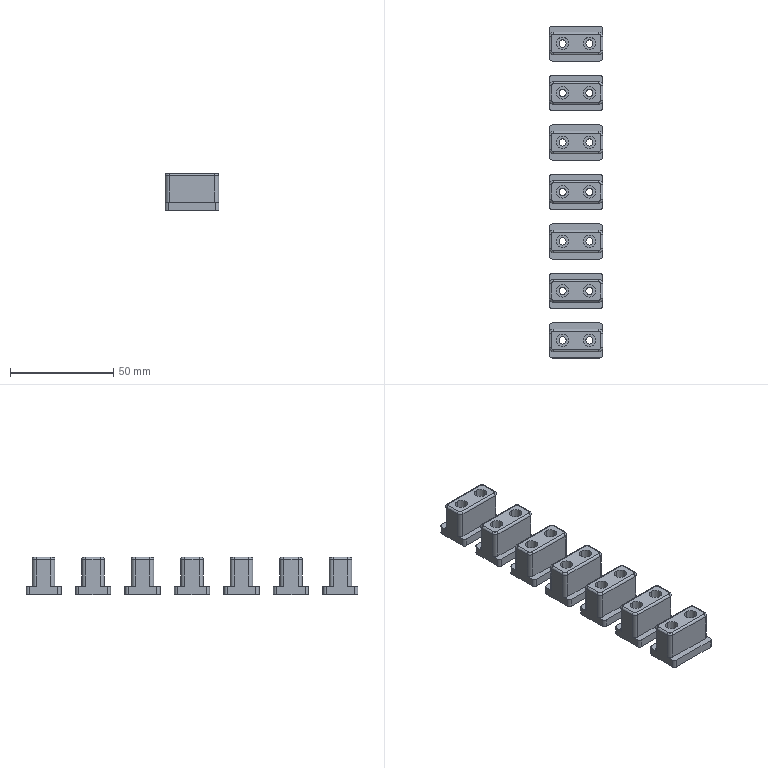NC program | NX | posted with a generic post | part box 26 x 161 x 18 mm
Whole program:
N10 G17 G21 G94 G90
(FLOOR_WALL_COPY , TOOL : D63)
N12 T01 M6
N14 G54
N16 G17 G0 G90 X-115. Y0. S6500 M3
N18 G43 Z30. H1
N20 Z9.
N22 G94 G1 Z6. F1250.
N24 X-112.
N26 X112.
N28 X115.
N30 Z9.
N32 G0 Z30.
N34 X-115.
N36 Z8.
N38 G1 Z5.
N40 X-112.
N42 X112.
N44 X115.
N46 Z8.
N48 G0 Z30.
N50 X-115.
N52 Z7.
N54 G1 Z4.
N56 X-112.
N58 X112.
N60 X115.
N62 Z7.
N64 G0 Z30.
N66 X-115.
N68 Z6.
N70 G1 Z3.
N72 X-112.
N74 X112.
N76 X115.
N78 Z6.
N80 G0 Z30.
N82 X-115.
N84 Z5.
N86 G1 Z2.
N88 X-112.
N90 X112.
N92 X115.
N94 Z5.
N96 G0 Z30.
N98 X-115.
N100 Z4.
N102 G1 Z1.
N104 X-112.
N106 X112.
N108 X115.
N110 Z4.
N112 G0 Z30.
N114 X-115.
N116 Z3.
N118 G1 Z0.
N120 X-112.
N122 X112.
N124 X115.
N126 Z3.
N128 G0 Z30.
N130 M5
(ZLEVEL_PROFILE_1_COPY_1_COPY_COPY_COPY , TOOL : D4A45)
N132 T02 M6
N134 G54
N136 G17 G0 G90 X72. Y7.291 S9500 M3
N138 G43 Z30. H2
N140 Z1.
N142 G94 G1 Z-1. F1000.
N144 G3 X71.209 Y6.5 R0.791
N146 X72. Y7.291 R-0.791
N148 X71.654 Y7.091 R0.4
N150 G1 Z0.
N152 G0 Z30.
N154 X72. Y-7.291
N156 Z1.
N158 G1 Z-1.
N160 G3 X72.791 Y-6.5 R0.791
N162 X72. Y-7.291 R-0.791
N164 X72.346 Y-7.091 R0.4
N166 G1 Z0.
N168 G0 Z30.
N170 X24. Y-7.291
N172 Z1.
N174 G1 Z-1.
N176 G3 X24.791 Y-6.5 R0.791
N178 X24. Y-7.291 R-0.791
N180 X24.346 Y-7.091 R0.4
N182 G1 Z0.
N184 G0 Z30.
N186 X24. Y7.291
N188 Z1.
N190 G1 Z-1.
N192 G3 X23.209 Y6.5 R0.791
N194 X24. Y7.291 R-0.791
N196 X23.654 Y7.091 R0.4
N198 G1 Z0.
N200 G0 Z30.
N202 X0. Y-7.291
N204 Z1.
N206 G1 Z-1.
N208 G3 X0.791 Y-6.5 R0.791
N210 X0. Y-7.291 R-0.791
N212 X0.346 Y-7.091 R0.4
N214 G1 Z0.
N216 G0 Z30.
N218 X0. Y7.291
N220 Z1.
N222 G1 Z-1.
N224 G3 X-0.791 Y6.5 R0.791
N226 X0. Y7.291 R-0.791
N228 X-0.346 Y7.091 R0.4
N230 G1 Z0.
N232 G0 Z30.
N234 X-24. Y-7.291
N236 Z1.
N238 G1 Z-1.
N240 G3 X-23.209 Y-6.5 R0.791
N242 X-24. Y-7.291 R-0.791
N244 X-23.654 Y-7.091 R0.4
N246 G1 Z0.
N248 G0 Z30.
N250 X-24. Y7.291
N252 Z1.
N254 G1 Z-1.
N256 G3 X-24.791 Y6.5 R0.791
N258 X-24. Y7.291 R-0.791
N260 X-24.346 Y7.091 R0.4
N262 G1 Z0.
N264 G0 Z30.
N266 X48. Y-7.291
N268 Z1.
N270 G1 Z-1.
N272 G3 X48.791 Y-6.5 R0.791
N274 X48. Y-7.291 R-0.791
N276 X48.346 Y-7.091 R0.4
N278 G1 Z0.
N280 G0 Z30.
N282 X48. Y7.291
N284 Z1.
N286 G1 Z-1.
N288 G3 X47.209 Y6.5 R0.791
N290 X48. Y7.291 R-0.791
N292 X47.654 Y7.091 R0.4
N294 G1 Z0.
N296 G0 Z30.
N298 X-48. Y-7.291
N300 Z1.
N302 G1 Z-1.
N304 G3 X-47.209 Y-6.5 R0.791
N306 X-48. Y-7.291 R-0.791
N308 X-47.654 Y-7.091 R0.4
N310 G1 Z0.
N312 G0 Z30.
N314 X-48. Y7.291
N316 Z1.
N318 G1 Z-1.
N320 G3 X-48.791 Y6.5 R0.791
N322 X-48. Y7.291 R-0.791
N324 X-48.346 Y7.091 R0.4
N326 G1 Z0.
N328 G0 Z30.
N330 X-72. Y-7.291
N332 Z1.
N334 G1 Z-1.
N336 G3 X-71.209 Y-6.5 R0.791
N338 X-72. Y-7.291 R-0.791
N340 X-71.654 Y-7.091 R0.4
N342 G1 Z0.
N344 G0 Z30.
N346 X-72. Y7.291
N348 Z1.
N350 G1 Z-1.
N352 G3 X-72.791 Y6.5 R0.791
N354 X-72. Y7.291 R-0.791
N356 X-72.346 Y7.091 R0.4
N358 G1 Z0.
N360 G0 Z30.
N362 X-82.192 Y-12.154
N364 Z0.
N366 G1 Z-1.
N368 X-81.659 Y-11.846
N370 G3 X-81.459 Y-11.5 R0.4
N372 G1 Y11.5
N374 G2 X-79. Y13.959 R2.459
N376 G1 X-65.
N378 G2 X-62.541 Y11.5 R2.459
N380 G1 Y-11.5
N382 G2 X-65. Y-13.959 R2.459
N384 G1 X-79.
N386 G2 X-81.459 Y-11.5 R2.459
N388 G3 X-81.659 Y-11.154 R0.4
N390 G1 X-82.259 Y-10.807
N392 Z0.
N394 G0 Z30.
N396 X-58.192 Y-12.154
N398 Z0.
N400 G1 Z-1.
N402 X-57.659 Y-11.846
N404 G3 X-57.459 Y-11.5 R0.4
N406 G1 Y11.5
N408 G2 X-55. Y13.959 R2.459
N410 G1 X-41.
N412 G2 X-38.541 Y11.5 R2.459
N414 G1 Y-11.5
N416 G2 X-41. Y-13.959 R2.459
N418 G1 X-55.
N420 G2 X-57.459 Y-11.5 R2.459
N422 G3 X-57.659 Y-11.154 R0.4
N424 G1 X-58.259 Y-10.807
N426 Z0.
N428 G0 Z30.
N430 X37.808 Y-12.154
N432 Z0.
N434 G1 Z-1.
N436 X38.341 Y-11.846
N438 G3 X38.541 Y-11.5 R0.4
N440 G1 Y11.5
N442 G2 X41. Y13.959 R2.459
N444 G1 X55.
N446 G2 X57.459 Y11.5 R2.459
N448 G1 Y-11.5
N450 G2 X55. Y-13.959 R2.459
N452 G1 X41.
N454 G2 X38.541 Y-11.5 R2.459
N456 G3 X38.341 Y-11.154 R0.4
N458 G1 X37.741 Y-10.807
N460 Z0.
N462 G0 Z30.
N464 X-13.808 Y12.154
N466 Z0.
N468 G1 Z-1.
N470 X-14.341 Y11.846
N472 G3 X-14.541 Y11.5 R0.4
N474 G1 Y-11.5
N476 G2 X-17. Y-13.959 R2.459
N478 G1 X-31.
N480 G2 X-33.459 Y-11.5 R2.459
N482 G1 Y11.5
N484 G2 X-31. Y13.959 R2.459
N486 G1 X-17.
N488 G2 X-14.541 Y11.5 R2.459
N490 G3 X-14.341 Y11.154 R0.4
N492 G1 X-13.741 Y10.807
N494 Z0.
N496 G0 Z30.
N498 X-10.192 Y-12.154
N500 Z0.
N502 G1 Z-1.
N504 X-9.659 Y-11.846
N506 G3 X-9.459 Y-11.5 R0.4
N508 G1 Y11.5
N510 G2 X-7. Y13.959 R2.459
N512 G1 X7.
N514 G2 X9.459 Y11.5 R2.459
N516 G1 Y-11.5
N518 G2 X7. Y-13.959 R2.459
N520 G1 X-7.
N522 G2 X-9.459 Y-11.5 R2.459
N524 G3 X-9.659 Y-11.154 R0.4
N526 G1 X-10.259 Y-10.807
N528 Z0.
N530 G0 Z30.
N532 X13.808 Y-12.154
N534 Z0.
N536 G1 Z-1.
N538 X14.341 Y-11.846
N540 G3 X14.541 Y-11.5 R0.4
N542 G1 Y11.5
N544 G2 X17. Y13.959 R2.459
N546 G1 X31.
N548 G2 X33.459 Y11.5 R2.459
N550 G1 Y-11.5
N552 G2 X31. Y-13.959 R2.459
N554 G1 X17.
N556 G2 X14.541 Y-11.5 R2.459
N558 G3 X14.341 Y-11.154 R0.4
N560 G1 X13.741 Y-10.807
N562 Z0.
N564 G0 Z30.
N566 X82.192 Y12.154
N568 Z0.
N570 G1 Z-1.
N572 X81.659 Y11.846
N574 G3 X81.459 Y11.5 R0.4
N576 G1 Y-11.5
N578 G2 X79. Y-13.959 R2.459
N580 G1 X65.
N582 G2 X62.541 Y-11.5 R2.459
N584 G1 Y11.5
N586 G2 X65. Y13.959 R2.459
N588 G1 X79.
N590 G2 X81.459 Y11.5 R2.459
N592 G3 X81.659 Y11.154 R0.4
N594 G1 X82.259 Y10.807
N596 Z0.
N598 G0 Z30.
N600 M5
N602 M2